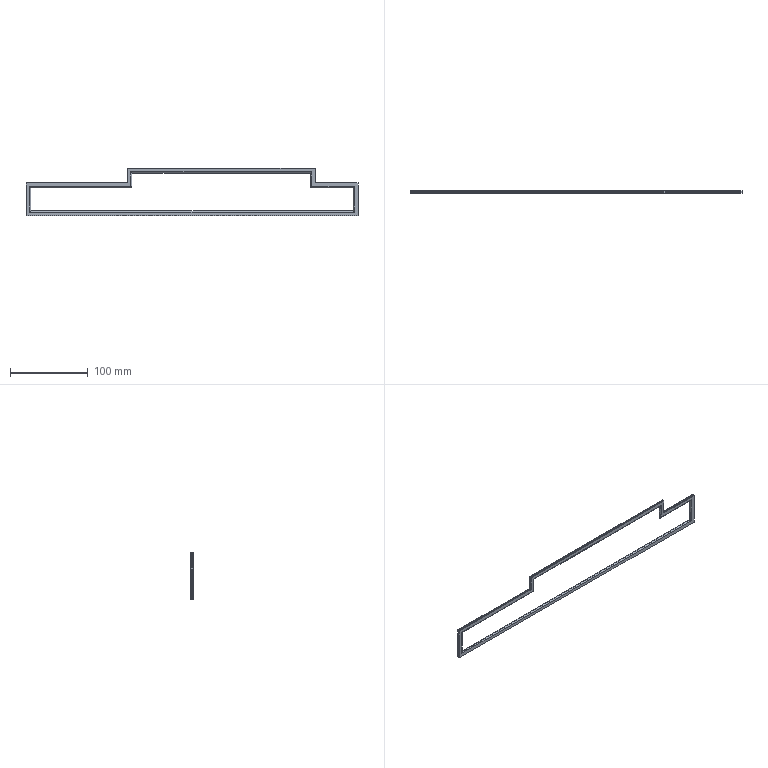Part | STEP file | _2000 | 1 solid | 36 faces | box 426.4 x 3 x 60.8 mm | volume 11438 mm3 | plane 28 | cylinder 8 | commonest cylinder face diameters 3 x8